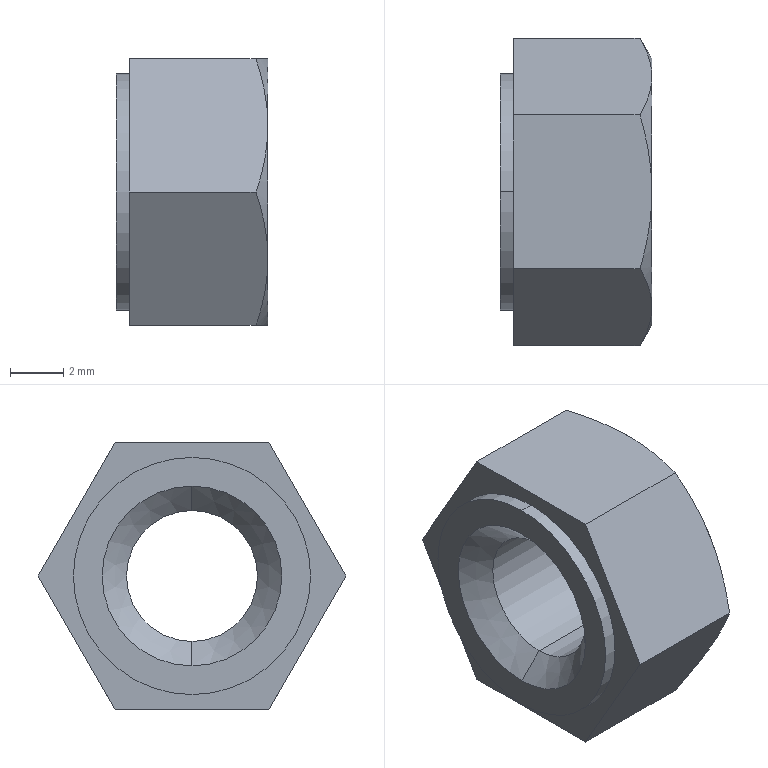Part | STEP file | Cut-Extrude 3-12 | 1 solid | 23 faces | box 5.7 x 11.547 x 10 mm | volume 357.503 mm3 | cone 10 | plane 9 | cylinder 4 | commonest cylinder face diameters 4.918 x2 8.9 x2
STEP:
#1=CARTESIAN_POINT('',(-1338.238,1764.264,2607.95));
#2=VERTEX_POINT('',#1);
#3=CARTESIAN_POINT('',(-1338.238,1764.264,2599.05));
#4=VERTEX_POINT('',#3);
#5=CARTESIAN_POINT('',(-1338.238,1764.264,2603.5));
#6=DIRECTION('',(-1.,0.,0.));
#7=DIRECTION('',(0.,0.,1.));
#8=AXIS2_PLACEMENT_3D('',#5,#6,#7);
#9=CIRCLE('',#8,4.45);
#10=EDGE_CURVE('',#2,#4,#9,.T.);
#11=ORIENTED_EDGE('',*,*,#10,.T.);
#12=CARTESIAN_POINT('',(-1338.738,1764.264,2599.05));
#13=VERTEX_POINT('',#12);
#14=CARTESIAN_POINT('',(-1338.238,1764.264,2599.05));
#15=DIRECTION('',(-1.,0.,0.));
#16=VECTOR('',#15,1000.);
#17=LINE('',#14,#16);
#18=EDGE_CURVE('',#4,#13,#17,.T.);
#19=ORIENTED_EDGE('',*,*,#18,.T.);
#20=CARTESIAN_POINT('',(-1338.738,1764.264,2607.95));
#21=VERTEX_POINT('',#20);
#22=CARTESIAN_POINT('',(-1338.738,1764.264,2603.5));
#23=DIRECTION('',(-1.,0.,0.));
#24=DIRECTION('',(0.,0.,1.));
#25=AXIS2_PLACEMENT_3D('',#22,#23,#24);
#26=CIRCLE('',#25,4.45);
#27=EDGE_CURVE('',#21,#13,#26,.T.);
#28=ORIENTED_EDGE('',*,*,#27,.F.);
#29=CARTESIAN_POINT('',(-1338.238,1764.264,2607.95));
#30=DIRECTION('',(-1.,0.,0.));
#31=VECTOR('',#30,1000.);
#32=LINE('',#29,#31);
#33=EDGE_CURVE('',#2,#21,#32,.T.);
#34=ORIENTED_EDGE('',*,*,#33,.F.);
#35=EDGE_LOOP('',(#11,#19,#28,#34));
#36=FACE_OUTER_BOUND('',#35,.T.);
#37=CARTESIAN_POINT('',(-1338.238,1764.264,2603.5));
#38=DIRECTION('',(-1.,0.,0.));
#39=DIRECTION('',(0.,0.,-1.));
#40=AXIS2_PLACEMENT_3D('',#37,#38,#39);
#41=CYLINDRICAL_SURFACE('',#40,4.45);
#42=ADVANCED_FACE('',(#36),#41,.T.);
#43=CARTESIAN_POINT('',(-1337.822,1764.264,2601.041));
#44=VERTEX_POINT('',#43);
#45=CARTESIAN_POINT('',(-1337.822,1764.264,2605.959));
#46=VERTEX_POINT('',#45);
#47=CARTESIAN_POINT('',(-1337.822,1764.264,2603.5));
#48=DIRECTION('',(-1.,0.,0.));
#49=DIRECTION('',(0.,0.,-1.));
#50=AXIS2_PLACEMENT_3D('',#47,#48,#49);
#51=CIRCLE('',#50,2.459);
#52=EDGE_CURVE('',#44,#46,#51,.T.);
#53=ORIENTED_EDGE('',*,*,#52,.F.);
#54=CARTESIAN_POINT('',(-1338.738,1764.264,2600.125));
#55=VERTEX_POINT('',#54);
#56=CARTESIAN_POINT('',(-1337.822,1764.264,2601.041));
#57=DIRECTION('',(-0.7071,0.,-0.7071));
#58=VECTOR('',#57,1000.);
#59=LINE('',#56,#58);
#60=EDGE_CURVE('',#44,#55,#59,.T.);
#61=ORIENTED_EDGE('',*,*,#60,.T.);
#62=CARTESIAN_POINT('',(-1338.738,1764.264,2606.875));
#63=VERTEX_POINT('',#62);
#64=CARTESIAN_POINT('',(-1338.738,1764.264,2603.5));
#65=DIRECTION('',(1.,0.,0.));
#66=DIRECTION('',(0.,0.,-1.));
#67=AXIS2_PLACEMENT_3D('',#64,#65,#66);
#68=CIRCLE('',#67,3.375);
#69=EDGE_CURVE('',#63,#55,#68,.T.);
#70=ORIENTED_EDGE('',*,*,#69,.F.);
#71=CARTESIAN_POINT('',(-1337.822,1764.264,2605.959));
#72=DIRECTION('',(-0.7071,0.,0.7071));
#73=VECTOR('',#72,1000.);
#74=LINE('',#71,#73);
#75=EDGE_CURVE('',#46,#63,#74,.T.);
#76=ORIENTED_EDGE('',*,*,#75,.F.);
#77=EDGE_LOOP('',(#53,#61,#70,#76));
#78=FACE_OUTER_BOUND('',#77,.T.);
#79=CARTESIAN_POINT('',(-1337.822,1764.264,2603.5));
#80=DIRECTION('',(-1.,0.,0.));
#81=DIRECTION('',(0.,0.,-1.));
#82=AXIS2_PLACEMENT_3D('',#79,#80,#81);
#83=CONICAL_SURFACE('',#82,2.459,0.7854);
#84=ADVANCED_FACE('',(#78),#83,.F.);
#85=CARTESIAN_POINT('',(-1333.955,1764.264,2605.959));
#86=VERTEX_POINT('',#85);
#87=CARTESIAN_POINT('',(-1333.955,1764.264,2601.041));
#88=VERTEX_POINT('',#87);
#89=CARTESIAN_POINT('',(-1333.955,1764.264,2603.5));
#90=DIRECTION('',(1.,0.,0.));
#91=DIRECTION('',(0.,0.,-1.));
#92=AXIS2_PLACEMENT_3D('',#89,#90,#91);
#93=CIRCLE('',#92,2.459);
#94=EDGE_CURVE('',#86,#88,#93,.T.);
#95=ORIENTED_EDGE('',*,*,#94,.F.);
#96=CARTESIAN_POINT('',(-1333.038,1764.264,2606.875));
#97=VERTEX_POINT('',#96);
#98=CARTESIAN_POINT('',(-1333.038,1764.264,2606.875));
#99=DIRECTION('',(-0.7071,0.,-0.7071));
#100=VECTOR('',#99,1000.);
#101=LINE('',#98,#100);
#102=EDGE_CURVE('',#97,#86,#101,.T.);
#103=ORIENTED_EDGE('',*,*,#102,.F.);
#104=CARTESIAN_POINT('',(-1333.038,1764.264,2600.125));
#105=VERTEX_POINT('',#104);
#106=CARTESIAN_POINT('',(-1333.038,1764.264,2603.5));
#107=DIRECTION('',(-1.,0.,0.));
#108=DIRECTION('',(0.,0.,-1.));
#109=AXIS2_PLACEMENT_3D('',#106,#107,#108);
#110=CIRCLE('',#109,3.375);
#111=EDGE_CURVE('',#105,#97,#110,.T.);
#112=ORIENTED_EDGE('',*,*,#111,.F.);
#113=CARTESIAN_POINT('',(-1333.038,1764.264,2600.125));
#114=DIRECTION('',(-0.7071,0.,0.7071));
#115=VECTOR('',#114,1000.);
#116=LINE('',#113,#115);
#117=EDGE_CURVE('',#105,#88,#116,.T.);
#118=ORIENTED_EDGE('',*,*,#117,.T.);
#119=EDGE_LOOP('',(#95,#103,#112,#118));
#120=FACE_OUTER_BOUND('',#119,.T.);
#121=CARTESIAN_POINT('',(-1333.038,1764.264,2603.5));
#122=DIRECTION('',(1.,0.,0.));
#123=DIRECTION('',(0.,0.,1.));
#124=AXIS2_PLACEMENT_3D('',#121,#122,#123);
#125=CONICAL_SURFACE('',#124,3.375,0.7854);
#126=ADVANCED_FACE('',(#120),#125,.F.);
#127=ORIENTED_EDGE('',*,*,#52,.T.);
#128=CARTESIAN_POINT('',(-1338.738,1764.264,2605.959));
#129=DIRECTION('',(-1.,0.,0.));
#130=VECTOR('',#129,1000.);
#131=LINE('',#128,#130);
#132=EDGE_CURVE('',#86,#46,#131,.T.);
#133=ORIENTED_EDGE('',*,*,#132,.F.);
#134=ORIENTED_EDGE('',*,*,#94,.T.);
#135=CARTESIAN_POINT('',(-1338.738,1764.264,2601.041));
#136=DIRECTION('',(-1.,0.,0.));
#137=VECTOR('',#136,1000.);
#138=LINE('',#135,#137);
#139=EDGE_CURVE('',#88,#44,#138,.T.);
#140=ORIENTED_EDGE('',*,*,#139,.T.);
#141=EDGE_LOOP('',(#127,#133,#134,#140));
#142=FACE_OUTER_BOUND('',#141,.T.);
#143=CARTESIAN_POINT('',(-1338.738,1764.264,2603.5));
#144=DIRECTION('',(1.,0.,0.));
#145=DIRECTION('',(0.,0.,1.));
#146=AXIS2_PLACEMENT_3D('',#143,#144,#145);
#147=CYLINDRICAL_SURFACE('',#146,2.459);
#148=ADVANCED_FACE('',(#142),#147,.F.);
#149=CARTESIAN_POINT('',(-1338.238,1767.151,2608.5));
#150=VERTEX_POINT('',#149);
#151=CARTESIAN_POINT('',(-1338.238,1770.038,2603.5));
#152=VERTEX_POINT('',#151);
#153=CARTESIAN_POINT('',(-1338.238,1767.151,2608.5));
#154=DIRECTION('',(0.,0.5,-0.866));
#155=VECTOR('',#154,1000.);
#156=LINE('',#153,#155);
#157=EDGE_CURVE('',#150,#152,#156,.T.);
#158=ORIENTED_EDGE('',*,*,#157,.F.);
#159=CARTESIAN_POINT('',(-1333.485,1767.151,2608.5));
#160=VERTEX_POINT('',#159);
#161=CARTESIAN_POINT('',(-1338.738,1767.151,2608.5));
#162=DIRECTION('',(1.,0.,0.));
#163=VECTOR('',#162,1000.);
#164=LINE('',#161,#163);
#165=EDGE_CURVE('',#150,#160,#164,.T.);
#166=ORIENTED_EDGE('',*,*,#165,.T.);
#167=CARTESIAN_POINT('',(-1333.038,1768.594,2606.));
#168=VERTEX_POINT('',#167);
#169=CARTESIAN_POINT('',(-1333.038,1768.594,2606.));
#170=CARTESIAN_POINT('',(-1333.038,1768.102,2606.853));
#171=CARTESIAN_POINT('',(-1333.213,1767.623,2607.683));
#172=CARTESIAN_POINT('',(-1333.485,1767.151,2608.5));
#173=B_SPLINE_CURVE_WITH_KNOTS('',3,(#169,#170,#171,#172),.UNSPECIFIED.,.F.,.F.,(4,4),(0.,0.002921),.UNSPECIFIED.);
#174=EDGE_CURVE('',#168,#160,#173,.T.);
#175=ORIENTED_EDGE('',*,*,#174,.F.);
#176=CARTESIAN_POINT('',(-1333.485,1770.038,2603.5));
#177=VERTEX_POINT('',#176);
#178=CARTESIAN_POINT('',(-1333.485,1770.038,2603.5));
#179=CARTESIAN_POINT('',(-1333.213,1769.566,2604.317));
#180=CARTESIAN_POINT('',(-1333.038,1769.087,2605.147));
#181=CARTESIAN_POINT('',(-1333.038,1768.594,2606.));
#182=B_SPLINE_CURVE_WITH_KNOTS('',3,(#178,#179,#180,#181),.UNSPECIFIED.,.F.,.F.,(4,4),(0.,0.002921),.UNSPECIFIED.);
#183=EDGE_CURVE('',#177,#168,#182,.T.);
#184=ORIENTED_EDGE('',*,*,#183,.F.);
#185=CARTESIAN_POINT('',(-1338.738,1770.038,2603.5));
#186=DIRECTION('',(1.,0.,0.));
#187=VECTOR('',#186,1000.);
#188=LINE('',#185,#187);
#189=EDGE_CURVE('',#152,#177,#188,.T.);
#190=ORIENTED_EDGE('',*,*,#189,.F.);
#191=EDGE_LOOP('',(#158,#166,#175,#184,#190));
#192=FACE_OUTER_BOUND('',#191,.T.);
#193=CARTESIAN_POINT('',(-1338.738,1767.151,2608.5));
#194=DIRECTION('',(0.,-0.866,-0.5));
#195=DIRECTION('',(0.,0.5,-0.866));
#196=AXIS2_PLACEMENT_3D('',#193,#194,#195);
#197=PLANE('',#196);
#198=ADVANCED_FACE('',(#192),#197,.F.);
#199=CARTESIAN_POINT('',(-1338.238,1767.151,2598.5));
#200=VERTEX_POINT('',#199);
#201=CARTESIAN_POINT('',(-1338.238,1770.038,2603.5));
#202=DIRECTION('',(0.,-0.5,-0.866));
#203=VECTOR('',#202,1000.);
#204=LINE('',#201,#203);
#205=EDGE_CURVE('',#152,#200,#204,.T.);
#206=ORIENTED_EDGE('',*,*,#205,.F.);
#207=ORIENTED_EDGE('',*,*,#189,.T.);
#208=CARTESIAN_POINT('',(-1333.038,1768.594,2601.));
#209=VERTEX_POINT('',#208);
#210=CARTESIAN_POINT('',(-1333.038,1768.594,2601.));
#211=CARTESIAN_POINT('',(-1333.038,1769.087,2601.853));
#212=CARTESIAN_POINT('',(-1333.213,1769.566,2602.683));
#213=CARTESIAN_POINT('',(-1333.485,1770.038,2603.5));
#214=B_SPLINE_CURVE_WITH_KNOTS('',3,(#210,#211,#212,#213),.UNSPECIFIED.,.F.,.F.,(4,4),(0.,0.002921),.UNSPECIFIED.);
#215=EDGE_CURVE('',#209,#177,#214,.T.);
#216=ORIENTED_EDGE('',*,*,#215,.F.);
#217=CARTESIAN_POINT('',(-1333.485,1767.151,2598.5));
#218=VERTEX_POINT('',#217);
#219=CARTESIAN_POINT('',(-1333.485,1767.151,2598.5));
#220=CARTESIAN_POINT('',(-1333.213,1767.623,2599.317));
#221=CARTESIAN_POINT('',(-1333.038,1768.102,2600.147));
#222=CARTESIAN_POINT('',(-1333.038,1768.594,2601.));
#223=B_SPLINE_CURVE_WITH_KNOTS('',3,(#219,#220,#221,#222),.UNSPECIFIED.,.F.,.F.,(4,4),(0.,0.002921),.UNSPECIFIED.);
#224=EDGE_CURVE('',#218,#209,#223,.T.);
#225=ORIENTED_EDGE('',*,*,#224,.F.);
#226=CARTESIAN_POINT('',(-1338.738,1767.151,2598.5));
#227=DIRECTION('',(1.,0.,0.));
#228=VECTOR('',#227,1000.);
#229=LINE('',#226,#228);
#230=EDGE_CURVE('',#200,#218,#229,.T.);
#231=ORIENTED_EDGE('',*,*,#230,.F.);
#232=EDGE_LOOP('',(#206,#207,#216,#225,#231));
#233=FACE_OUTER_BOUND('',#232,.T.);
#234=CARTESIAN_POINT('',(-1338.738,1770.038,2603.5));
#235=DIRECTION('',(0.,-0.866,0.5));
#236=DIRECTION('',(0.,-0.5,-0.866));
#237=AXIS2_PLACEMENT_3D('',#234,#235,#236);
#238=PLANE('',#237);
#239=ADVANCED_FACE('',(#233),#238,.F.);
#240=CARTESIAN_POINT('',(-1338.238,1761.378,2598.5));
#241=VERTEX_POINT('',#240);
#242=CARTESIAN_POINT('',(-1338.238,1767.151,2598.5));
#243=DIRECTION('',(0.,-1.,0.));
#244=VECTOR('',#243,1000.);
#245=LINE('',#242,#244);
#246=EDGE_CURVE('',#200,#241,#245,.T.);
#247=ORIENTED_EDGE('',*,*,#246,.F.);
#248=ORIENTED_EDGE('',*,*,#230,.T.);
#249=CARTESIAN_POINT('',(-1333.038,1764.264,2598.5));
#250=VERTEX_POINT('',#249);
#251=CARTESIAN_POINT('',(-1333.038,1764.264,2598.5));
#252=CARTESIAN_POINT('',(-1333.038,1765.25,2598.5));
#253=CARTESIAN_POINT('',(-1333.213,1766.208,2598.5));
#254=CARTESIAN_POINT('',(-1333.485,1767.151,2598.5));
#255=B_SPLINE_CURVE_WITH_KNOTS('',3,(#251,#252,#253,#254),.UNSPECIFIED.,.F.,.F.,(4,4),(0.,0.002921),.UNSPECIFIED.);
#256=EDGE_CURVE('',#250,#218,#255,.T.);
#257=ORIENTED_EDGE('',*,*,#256,.F.);
#258=CARTESIAN_POINT('',(-1333.485,1761.378,2598.5));
#259=VERTEX_POINT('',#258);
#260=CARTESIAN_POINT('',(-1333.485,1761.378,2598.5));
#261=CARTESIAN_POINT('',(-1333.213,1762.321,2598.5));
#262=CARTESIAN_POINT('',(-1333.038,1763.279,2598.5));
#263=CARTESIAN_POINT('',(-1333.038,1764.264,2598.5));
#264=B_SPLINE_CURVE_WITH_KNOTS('',3,(#260,#261,#262,#263),.UNSPECIFIED.,.F.,.F.,(4,4),(0.,0.002921),.UNSPECIFIED.);
#265=EDGE_CURVE('',#259,#250,#264,.T.);
#266=ORIENTED_EDGE('',*,*,#265,.F.);
#267=CARTESIAN_POINT('',(-1338.738,1761.378,2598.5));
#268=DIRECTION('',(1.,0.,0.));
#269=VECTOR('',#268,1000.);
#270=LINE('',#267,#269);
#271=EDGE_CURVE('',#241,#259,#270,.T.);
#272=ORIENTED_EDGE('',*,*,#271,.F.);
#273=EDGE_LOOP('',(#247,#248,#257,#266,#272));
#274=FACE_OUTER_BOUND('',#273,.T.);
#275=CARTESIAN_POINT('',(-1338.738,1767.151,2598.5));
#276=DIRECTION('',(0.,0.,1.));
#277=DIRECTION('',(0.,-1.,0.));
#278=AXIS2_PLACEMENT_3D('',#275,#276,#277);
#279=PLANE('',#278);
#280=ADVANCED_FACE('',(#274),#279,.F.);
#281=CARTESIAN_POINT('',(-1338.238,1758.491,2603.5));
#282=VERTEX_POINT('',#281);
#283=CARTESIAN_POINT('',(-1338.238,1761.378,2598.5));
#284=DIRECTION('',(0.,-0.5,0.866));
#285=VECTOR('',#284,1000.);
#286=LINE('',#283,#285);
#287=EDGE_CURVE('',#241,#282,#286,.T.);
#288=ORIENTED_EDGE('',*,*,#287,.F.);
#289=ORIENTED_EDGE('',*,*,#271,.T.);
#290=CARTESIAN_POINT('',(-1333.038,1759.934,2601.));
#291=VERTEX_POINT('',#290);
#292=CARTESIAN_POINT('',(-1333.038,1759.934,2601.));
#293=CARTESIAN_POINT('',(-1333.038,1760.427,2600.147));
#294=CARTESIAN_POINT('',(-1333.213,1760.906,2599.317));
#295=CARTESIAN_POINT('',(-1333.485,1761.378,2598.5));
#296=B_SPLINE_CURVE_WITH_KNOTS('',3,(#292,#293,#294,#295),.UNSPECIFIED.,.F.,.F.,(4,4),(0.,0.002921),.UNSPECIFIED.);
#297=EDGE_CURVE('',#291,#259,#296,.T.);
#298=ORIENTED_EDGE('',*,*,#297,.F.);
#299=CARTESIAN_POINT('',(-1333.485,1758.491,2603.5));
#300=VERTEX_POINT('',#299);
#301=CARTESIAN_POINT('',(-1333.485,1758.491,2603.5));
#302=CARTESIAN_POINT('',(-1333.213,1758.962,2602.683));
#303=CARTESIAN_POINT('',(-1333.038,1759.442,2601.853));
#304=CARTESIAN_POINT('',(-1333.038,1759.934,2601.));
#305=B_SPLINE_CURVE_WITH_KNOTS('',3,(#301,#302,#303,#304),.UNSPECIFIED.,.F.,.F.,(4,4),(0.,0.002921),.UNSPECIFIED.);
#306=EDGE_CURVE('',#300,#291,#305,.T.);
#307=ORIENTED_EDGE('',*,*,#306,.F.);
#308=CARTESIAN_POINT('',(-1338.738,1758.491,2603.5));
#309=DIRECTION('',(1.,0.,0.));
#310=VECTOR('',#309,1000.);
#311=LINE('',#308,#310);
#312=EDGE_CURVE('',#282,#300,#311,.T.);
#313=ORIENTED_EDGE('',*,*,#312,.F.);
#314=EDGE_LOOP('',(#288,#289,#298,#307,#313));
#315=FACE_OUTER_BOUND('',#314,.T.);
#316=CARTESIAN_POINT('',(-1338.738,1761.378,2598.5));
#317=DIRECTION('',(0.,0.866,0.5));
#318=DIRECTION('',(0.,-0.5,0.866));
#319=AXIS2_PLACEMENT_3D('',#316,#317,#318);
#320=PLANE('',#319);
#321=ADVANCED_FACE('',(#315),#320,.F.);
#322=CARTESIAN_POINT('',(-1338.238,1761.378,2608.5));
#323=VERTEX_POINT('',#322);
#324=CARTESIAN_POINT('',(-1338.238,1758.491,2603.5));
#325=DIRECTION('',(0.,0.5,0.866));
#326=VECTOR('',#325,1000.);
#327=LINE('',#324,#326);
#328=EDGE_CURVE('',#282,#323,#327,.T.);
#329=ORIENTED_EDGE('',*,*,#328,.F.);
#330=ORIENTED_EDGE('',*,*,#312,.T.);
#331=CARTESIAN_POINT('',(-1333.038,1759.934,2606.));
#332=VERTEX_POINT('',#331);
#333=CARTESIAN_POINT('',(-1333.038,1759.934,2606.));
#334=CARTESIAN_POINT('',(-1333.038,1759.442,2605.147));
#335=CARTESIAN_POINT('',(-1333.213,1758.962,2604.317));
#336=CARTESIAN_POINT('',(-1333.485,1758.491,2603.5));
#337=B_SPLINE_CURVE_WITH_KNOTS('',3,(#333,#334,#335,#336),.UNSPECIFIED.,.F.,.F.,(4,4),(0.,0.002921),.UNSPECIFIED.);
#338=EDGE_CURVE('',#332,#300,#337,.T.);
#339=ORIENTED_EDGE('',*,*,#338,.F.);
#340=CARTESIAN_POINT('',(-1333.485,1761.378,2608.5));
#341=VERTEX_POINT('',#340);
#342=CARTESIAN_POINT('',(-1333.485,1761.378,2608.5));
#343=CARTESIAN_POINT('',(-1333.213,1760.906,2607.683));
#344=CARTESIAN_POINT('',(-1333.038,1760.427,2606.853));
#345=CARTESIAN_POINT('',(-1333.038,1759.934,2606.));
#346=B_SPLINE_CURVE_WITH_KNOTS('',3,(#342,#343,#344,#345),.UNSPECIFIED.,.F.,.F.,(4,4),(0.,0.002921),.UNSPECIFIED.);
#347=EDGE_CURVE('',#341,#332,#346,.T.);
#348=ORIENTED_EDGE('',*,*,#347,.F.);
#349=CARTESIAN_POINT('',(-1338.738,1761.378,2608.5));
#350=DIRECTION('',(1.,0.,0.));
#351=VECTOR('',#350,1000.);
#352=LINE('',#349,#351);
#353=EDGE_CURVE('',#323,#341,#352,.T.);
#354=ORIENTED_EDGE('',*,*,#353,.F.);
#355=EDGE_LOOP('',(#329,#330,#339,#348,#354));
#356=FACE_OUTER_BOUND('',#355,.T.);
#357=CARTESIAN_POINT('',(-1338.738,1758.491,2603.5));
#358=DIRECTION('',(0.,0.866,-0.5));
#359=DIRECTION('',(0.,0.5,0.866));
#360=AXIS2_PLACEMENT_3D('',#357,#358,#359);
#361=PLANE('',#360);
#362=ADVANCED_FACE('',(#356),#361,.F.);
#363=CARTESIAN_POINT('',(-1338.238,1761.378,2608.5));
#364=DIRECTION('',(0.,1.,0.));
#365=VECTOR('',#364,1000.);
#366=LINE('',#363,#365);
#367=EDGE_CURVE('',#323,#150,#366,.T.);
#368=ORIENTED_EDGE('',*,*,#367,.F.);
#369=ORIENTED_EDGE('',*,*,#353,.T.);
#370=CARTESIAN_POINT('',(-1333.038,1764.264,2608.5));
#371=VERTEX_POINT('',#370);
#372=CARTESIAN_POINT('',(-1333.038,1764.264,2608.5));
#373=CARTESIAN_POINT('',(-1333.038,1763.279,2608.5));
#374=CARTESIAN_POINT('',(-1333.213,1762.321,2608.5));
#375=CARTESIAN_POINT('',(-1333.485,1761.378,2608.5));
#376=B_SPLINE_CURVE_WITH_KNOTS('',3,(#372,#373,#374,#375),.UNSPECIFIED.,.F.,.F.,(4,4),(0.,0.002921),.UNSPECIFIED.);
#377=EDGE_CURVE('',#371,#341,#376,.T.);
#378=ORIENTED_EDGE('',*,*,#377,.F.);
#379=CARTESIAN_POINT('',(-1333.485,1767.151,2608.5));
#380=CARTESIAN_POINT('',(-1333.213,1766.208,2608.5));
#381=CARTESIAN_POINT('',(-1333.038,1765.25,2608.5));
#382=CARTESIAN_POINT('',(-1333.038,1764.264,2608.5));
#383=B_SPLINE_CURVE_WITH_KNOTS('',3,(#379,#380,#381,#382),.UNSPECIFIED.,.F.,.F.,(4,4),(0.,0.002921),.UNSPECIFIED.);
#384=EDGE_CURVE('',#160,#371,#383,.T.);
#385=ORIENTED_EDGE('',*,*,#384,.F.);
#386=ORIENTED_EDGE('',*,*,#165,.F.);
#387=EDGE_LOOP('',(#368,#369,#378,#385,#386));
#388=FACE_OUTER_BOUND('',#387,.T.);
#389=CARTESIAN_POINT('',(-1338.738,1761.378,2608.5));
#390=DIRECTION('',(0.,0.,-1.));
#391=DIRECTION('',(0.,1.,0.));
#392=AXIS2_PLACEMENT_3D('',#389,#390,#391);
#393=PLANE('',#392);
#394=ADVANCED_FACE('',(#388),#393,.F.);
#395=ORIENTED_EDGE('',*,*,#69,.T.);
#396=CARTESIAN_POINT('',(-1338.738,1764.264,2603.5));
#397=DIRECTION('',(1.,0.,0.));
#398=DIRECTION('',(0.,0.,-1.));
#399=AXIS2_PLACEMENT_3D('',#396,#397,#398);
#400=CIRCLE('',#399,3.375);
#401=EDGE_CURVE('',#55,#63,#400,.T.);
#402=ORIENTED_EDGE('',*,*,#401,.T.);
#403=EDGE_LOOP('',(#395,#402));
#404=FACE_BOUND('',#403,.T.);
#405=ORIENTED_EDGE('',*,*,#27,.T.);
#406=CARTESIAN_POINT('',(-1338.738,1764.264,2603.5));
#407=DIRECTION('',(-1.,0.,0.));
#408=DIRECTION('',(0.,0.,1.));
#409=AXIS2_PLACEMENT_3D('',#406,#407,#408);
#410=CIRCLE('',#409,4.45);
#411=EDGE_CURVE('',#13,#21,#410,.T.);
#412=ORIENTED_EDGE('',*,*,#411,.T.);
#413=EDGE_LOOP('',(#405,#412));
#414=FACE_OUTER_BOUND('',#413,.T.);
#415=CARTESIAN_POINT('',(-1338.738,1767.151,2608.5));
#416=DIRECTION('',(1.,0.,0.));
#417=DIRECTION('',(0.,0.,1.));
#418=AXIS2_PLACEMENT_3D('',#415,#416,#417);
#419=PLANE('',#418);
#420=ADVANCED_FACE('',(#404,#414),#419,.F.);
#421=ORIENTED_EDGE('',*,*,#111,.T.);
#422=CARTESIAN_POINT('',(-1333.038,1764.264,2603.5));
#423=DIRECTION('',(-1.,0.,0.));
#424=DIRECTION('',(0.,0.,-1.));
#425=AXIS2_PLACEMENT_3D('',#422,#423,#424);
#426=CIRCLE('',#425,3.375);
#427=EDGE_CURVE('',#97,#105,#426,.T.);
#428=ORIENTED_EDGE('',*,*,#427,.T.);
#429=EDGE_LOOP('',(#421,#428));
#430=FACE_BOUND('',#429,.T.);
#431=CARTESIAN_POINT('',(-1333.038,1764.264,2603.5));
#432=DIRECTION('',(1.,0.,0.));
#433=DIRECTION('',(0.,0.,-1.));
#434=AXIS2_PLACEMENT_3D('',#431,#432,#433);
#435=CIRCLE('',#434,5.);
#436=EDGE_CURVE('',#291,#250,#435,.T.);
#437=ORIENTED_EDGE('',*,*,#436,.T.);
#438=CARTESIAN_POINT('',(-1333.038,1764.264,2603.5));
#439=DIRECTION('',(1.,0.,0.));
#440=DIRECTION('',(0.,0.,-1.));
#441=AXIS2_PLACEMENT_3D('',#438,#439,#440);
#442=CIRCLE('',#441,5.);
#443=EDGE_CURVE('',#250,#209,#442,.T.);
#444=ORIENTED_EDGE('',*,*,#443,.T.);
#445=CARTESIAN_POINT('',(-1333.038,1764.264,2603.5));
#446=DIRECTION('',(1.,0.,0.));
#447=DIRECTION('',(0.,0.,-1.));
#448=AXIS2_PLACEMENT_3D('',#445,#446,#447);
#449=CIRCLE('',#448,5.);
#450=EDGE_CURVE('',#209,#168,#449,.T.);
#451=ORIENTED_EDGE('',*,*,#450,.T.);
#452=CARTESIAN_POINT('',(-1333.038,1764.264,2603.5));
#453=DIRECTION('',(1.,0.,0.));
#454=DIRECTION('',(0.,0.,-1.));
#455=AXIS2_PLACEMENT_3D('',#452,#453,#454);
#456=CIRCLE('',#455,5.);
#457=EDGE_CURVE('',#168,#371,#456,.T.);
#458=ORIENTED_EDGE('',*,*,#457,.T.);
#459=CARTESIAN_POINT('',(-1333.038,1764.264,2603.5));
#460=DIRECTION('',(1.,0.,0.));
#461=DIRECTION('',(0.,0.,-1.));
#462=AXIS2_PLACEMENT_3D('',#459,#460,#461);
#463=CIRCLE('',#462,5.);
#464=EDGE_CURVE('',#371,#332,#463,.T.);
#465=ORIENTED_EDGE('',*,*,#464,.T.);
#466=CARTESIAN_POINT('',(-1333.038,1764.264,2603.5));
#467=DIRECTION('',(1.,0.,0.));
#468=DIRECTION('',(0.,0.,-1.));
#469=AXIS2_PLACEMENT_3D('',#466,#467,#468);
#470=CIRCLE('',#469,5.);
#471=EDGE_CURVE('',#332,#291,#470,.T.);
#472=ORIENTED_EDGE('',*,*,#471,.T.);
#473=EDGE_LOOP('',(#437,#444,#451,#458,#465,#472));
#474=FACE_OUTER_BOUND('',#473,.T.);
#475=CARTESIAN_POINT('',(-1333.038,1767.151,2608.5));
#476=DIRECTION('',(1.,0.,0.));
#477=DIRECTION('',(0.,0.,1.));
#478=AXIS2_PLACEMENT_3D('',#475,#476,#477);
#479=PLANE('',#478);
#480=ADVANCED_FACE('',(#430,#474),#479,.T.);
#481=ORIENTED_EDGE('',*,*,#132,.T.);
#482=CARTESIAN_POINT('',(-1337.822,1764.264,2603.5));
#483=DIRECTION('',(-1.,0.,0.));
#484=DIRECTION('',(0.,0.,-1.));
#485=AXIS2_PLACEMENT_3D('',#482,#483,#484);
#486=CIRCLE('',#485,2.459);
#487=EDGE_CURVE('',#46,#44,#486,.T.);
#488=ORIENTED_EDGE('',*,*,#487,.T.);
#489=ORIENTED_EDGE('',*,*,#139,.F.);
#490=CARTESIAN_POINT('',(-1333.955,1764.264,2603.5));
#491=DIRECTION('',(1.,0.,0.));
#492=DIRECTION('',(0.,0.,-1.));
#493=AXIS2_PLACEMENT_3D('',#490,#491,#492);
#494=CIRCLE('',#493,2.459);
#495=EDGE_CURVE('',#88,#86,#494,.T.);
#496=ORIENTED_EDGE('',*,*,#495,.T.);
#497=EDGE_LOOP('',(#481,#488,#489,#496));
#498=FACE_OUTER_BOUND('',#497,.T.);
#499=CARTESIAN_POINT('',(-1338.738,1764.264,2603.5));
#500=DIRECTION('',(1.,0.,0.));
#501=DIRECTION('',(0.,0.,1.));
#502=AXIS2_PLACEMENT_3D('',#499,#500,#501);
#503=CYLINDRICAL_SURFACE('',#502,2.459);
#504=ADVANCED_FACE('',(#498),#503,.F.);
#505=ORIENTED_EDGE('',*,*,#347,.T.);
#506=ORIENTED_EDGE('',*,*,#464,.F.);
#507=ORIENTED_EDGE('',*,*,#377,.T.);
#508=EDGE_LOOP('',(#505,#506,#507));
#509=FACE_OUTER_BOUND('',#508,.T.);
#510=CARTESIAN_POINT('',(-1333.038,1764.264,2603.5));
#511=DIRECTION('',(-1.,0.,0.));
#512=DIRECTION('',(0.,0.,1.));
#513=AXIS2_PLACEMENT_3D('',#510,#511,#512);
#514=CONICAL_SURFACE('',#513,5.,1.047);
#515=ADVANCED_FACE('',(#509),#514,.T.);
#516=ORIENTED_EDGE('',*,*,#174,.T.);
#517=ORIENTED_EDGE('',*,*,#384,.T.);
#518=ORIENTED_EDGE('',*,*,#457,.F.);
#519=EDGE_LOOP('',(#516,#517,#518));
#520=FACE_OUTER_BOUND('',#519,.T.);
#521=CARTESIAN_POINT('',(-1333.038,1764.264,2603.5));
#522=DIRECTION('',(-1.,0.,0.));
#523=DIRECTION('',(0.,0.,1.));
#524=AXIS2_PLACEMENT_3D('',#521,#522,#523);
#525=CONICAL_SURFACE('',#524,5.,1.047);
#526=ADVANCED_FACE('',(#520),#525,.T.);
#527=ORIENTED_EDGE('',*,*,#306,.T.);
#528=ORIENTED_EDGE('',*,*,#471,.F.);
#529=ORIENTED_EDGE('',*,*,#338,.T.);
#530=EDGE_LOOP('',(#527,#528,#529));
#531=FACE_OUTER_BOUND('',#530,.T.);
#532=CARTESIAN_POINT('',(-1333.038,1764.264,2603.5));
#533=DIRECTION('',(-1.,0.,0.));
#534=DIRECTION('',(0.,0.,1.));
#535=AXIS2_PLACEMENT_3D('',#532,#533,#534);
#536=CONICAL_SURFACE('',#535,5.,1.047);
#537=ADVANCED_FACE('',(#531),#536,.T.);
#538=ORIENTED_EDGE('',*,*,#265,.T.);
#539=ORIENTED_EDGE('',*,*,#436,.F.);
#540=ORIENTED_EDGE('',*,*,#297,.T.);
#541=EDGE_LOOP('',(#538,#539,#540));
#542=FACE_OUTER_BOUND('',#541,.T.);
#543=CARTESIAN_POINT('',(-1333.038,1764.264,2603.5));
#544=DIRECTION('',(-1.,0.,0.));
#545=DIRECTION('',(0.,0.,1.));
#546=AXIS2_PLACEMENT_3D('',#543,#544,#545);
#547=CONICAL_SURFACE('',#546,5.,1.047);
#548=ADVANCED_FACE('',(#542),#547,.T.);
#549=ORIENTED_EDGE('',*,*,#256,.T.);
#550=ORIENTED_EDGE('',*,*,#224,.T.);
#551=ORIENTED_EDGE('',*,*,#443,.F.);
#552=EDGE_LOOP('',(#549,#550,#551));
#553=FACE_OUTER_BOUND('',#552,.T.);
#554=CARTESIAN_POINT('',(-1333.038,1764.264,2603.5));
#555=DIRECTION('',(-1.,0.,0.));
#556=DIRECTION('',(0.,0.,1.));
#557=AXIS2_PLACEMENT_3D('',#554,#555,#556);
#558=CONICAL_SURFACE('',#557,5.,1.047);
#559=ADVANCED_FACE('',(#553),#558,.T.);
#560=ORIENTED_EDGE('',*,*,#215,.T.);
#561=ORIENTED_EDGE('',*,*,#183,.T.);
#562=ORIENTED_EDGE('',*,*,#450,.F.);
#563=EDGE_LOOP('',(#560,#561,#562));
#564=FACE_OUTER_BOUND('',#563,.T.);
#565=CARTESIAN_POINT('',(-1333.038,1764.264,2603.5));
#566=DIRECTION('',(-1.,0.,0.));
#567=DIRECTION('',(0.,0.,1.));
#568=AXIS2_PLACEMENT_3D('',#565,#566,#567);
#569=CONICAL_SURFACE('',#568,5.,1.047);
#570=ADVANCED_FACE('',(#564),#569,.T.);
#571=ORIENTED_EDGE('',*,*,#102,.T.);
#572=ORIENTED_EDGE('',*,*,#495,.F.);
#573=ORIENTED_EDGE('',*,*,#117,.F.);
#574=ORIENTED_EDGE('',*,*,#427,.F.);
#575=EDGE_LOOP('',(#571,#572,#573,#574));
#576=FACE_OUTER_BOUND('',#575,.T.);
#577=CARTESIAN_POINT('',(-1333.038,1764.264,2603.5));
#578=DIRECTION('',(1.,0.,0.));
#579=DIRECTION('',(0.,0.,1.));
#580=AXIS2_PLACEMENT_3D('',#577,#578,#579);
#581=CONICAL_SURFACE('',#580,3.375,0.7854);
#582=ADVANCED_FACE('',(#576),#581,.F.);
#583=ORIENTED_EDGE('',*,*,#60,.F.);
#584=ORIENTED_EDGE('',*,*,#487,.F.);
#585=ORIENTED_EDGE('',*,*,#75,.T.);
#586=ORIENTED_EDGE('',*,*,#401,.F.);
#587=EDGE_LOOP('',(#583,#584,#585,#586));
#588=FACE_OUTER_BOUND('',#587,.T.);
#589=CARTESIAN_POINT('',(-1337.822,1764.264,2603.5));
#590=DIRECTION('',(-1.,0.,0.));
#591=DIRECTION('',(0.,0.,-1.));
#592=AXIS2_PLACEMENT_3D('',#589,#590,#591);
#593=CONICAL_SURFACE('',#592,2.459,0.7854);
#594=ADVANCED_FACE('',(#588),#593,.F.);
#595=ORIENTED_EDGE('',*,*,#10,.F.);
#596=CARTESIAN_POINT('',(-1338.238,1764.264,2603.5));
#597=DIRECTION('',(-1.,0.,0.));
#598=DIRECTION('',(0.,0.,1.));
#599=AXIS2_PLACEMENT_3D('',#596,#597,#598);
#600=CIRCLE('',#599,4.45);
#601=EDGE_CURVE('',#4,#2,#600,.T.);
#602=ORIENTED_EDGE('',*,*,#601,.F.);
#603=EDGE_LOOP('',(#595,#602));
#604=FACE_BOUND('',#603,.T.);
#605=ORIENTED_EDGE('',*,*,#157,.T.);
#606=ORIENTED_EDGE('',*,*,#205,.T.);
#607=ORIENTED_EDGE('',*,*,#246,.T.);
#608=ORIENTED_EDGE('',*,*,#287,.T.);
#609=ORIENTED_EDGE('',*,*,#328,.T.);
#610=ORIENTED_EDGE('',*,*,#367,.T.);
#611=EDGE_LOOP('',(#605,#606,#607,#608,#609,#610));
#612=FACE_OUTER_BOUND('',#611,.T.);
#613=CARTESIAN_POINT('',(-1338.238,1764.264,2603.5));
#614=DIRECTION('',(-1.,0.,0.));
#615=DIRECTION('',(0.,0.,-1.));
#616=AXIS2_PLACEMENT_3D('',#613,#614,#615);
#617=PLANE('',#616);
#618=ADVANCED_FACE('',(#604,#612),#617,.T.);
#619=ORIENTED_EDGE('',*,*,#18,.F.);
#620=ORIENTED_EDGE('',*,*,#601,.T.);
#621=ORIENTED_EDGE('',*,*,#33,.T.);
#622=ORIENTED_EDGE('',*,*,#411,.F.);
#623=EDGE_LOOP('',(#619,#620,#621,#622));
#624=FACE_OUTER_BOUND('',#623,.T.);
#625=CARTESIAN_POINT('',(-1338.238,1764.264,2603.5));
#626=DIRECTION('',(-1.,0.,0.));
#627=DIRECTION('',(0.,0.,-1.));
#628=AXIS2_PLACEMENT_3D('',#625,#626,#627);
#629=CYLINDRICAL_SURFACE('',#628,4.45);
#630=ADVANCED_FACE('',(#624),#629,.T.);
#631=CLOSED_SHELL('',(#42,#84,#126,#148,#198,#239,#280,#321,#362,#394,#420,#480,#504,#515,#526,#537,#548,#559,#570,#582,#594,#618,#630));
#632=MANIFOLD_SOLID_BREP('',#631);
#633=CARTESIAN_POINT('',(0.,0.,0.));
#634=DIRECTION('',(0.,0.,1.));
#635=DIRECTION('',(1.,0.,0.));
#636=AXIS2_PLACEMENT_3D('',#633,#634,#635);
#637=(LENGTH_UNIT()NAMED_UNIT(*)SI_UNIT(.MILLI.,.METRE.));
#638=UNCERTAINTY_MEASURE_WITH_UNIT(LENGTH_MEASURE(0.00001),#637,'','');
#639=(NAMED_UNIT(*)PLANE_ANGLE_UNIT()SI_UNIT($,.RADIAN.));
#640=(NAMED_UNIT(*)SI_UNIT($,.STERADIAN.)SOLID_ANGLE_UNIT());
#641=(GEOMETRIC_REPRESENTATION_CONTEXT(3)GLOBAL_UNCERTAINTY_ASSIGNED_CONTEXT((#638))GLOBAL_UNIT_ASSIGNED_CONTEXT((#637,#639,#640))REPRESENTATION_CONTEXT('',''));
#642=ADVANCED_BREP_SHAPE_REPRESENTATION('',(#632,#636),#641);